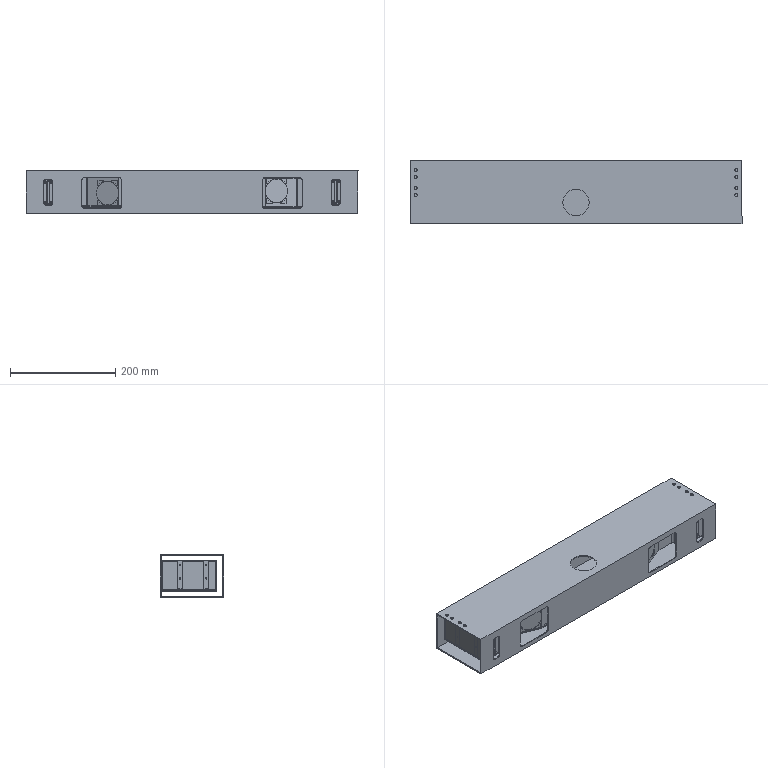Part | SolidWorks | 5 solids | 1556 faces | box 630 x 120 x 80 mm | volume 2553807 mm3 | plane 790 | cylinder 374 | spline 272 | cone 116 | torus 4 | commonest cylinder face diameters 2 x52 3 x40 4 x32 2.5 x28 1.6 x16 2.542 x16